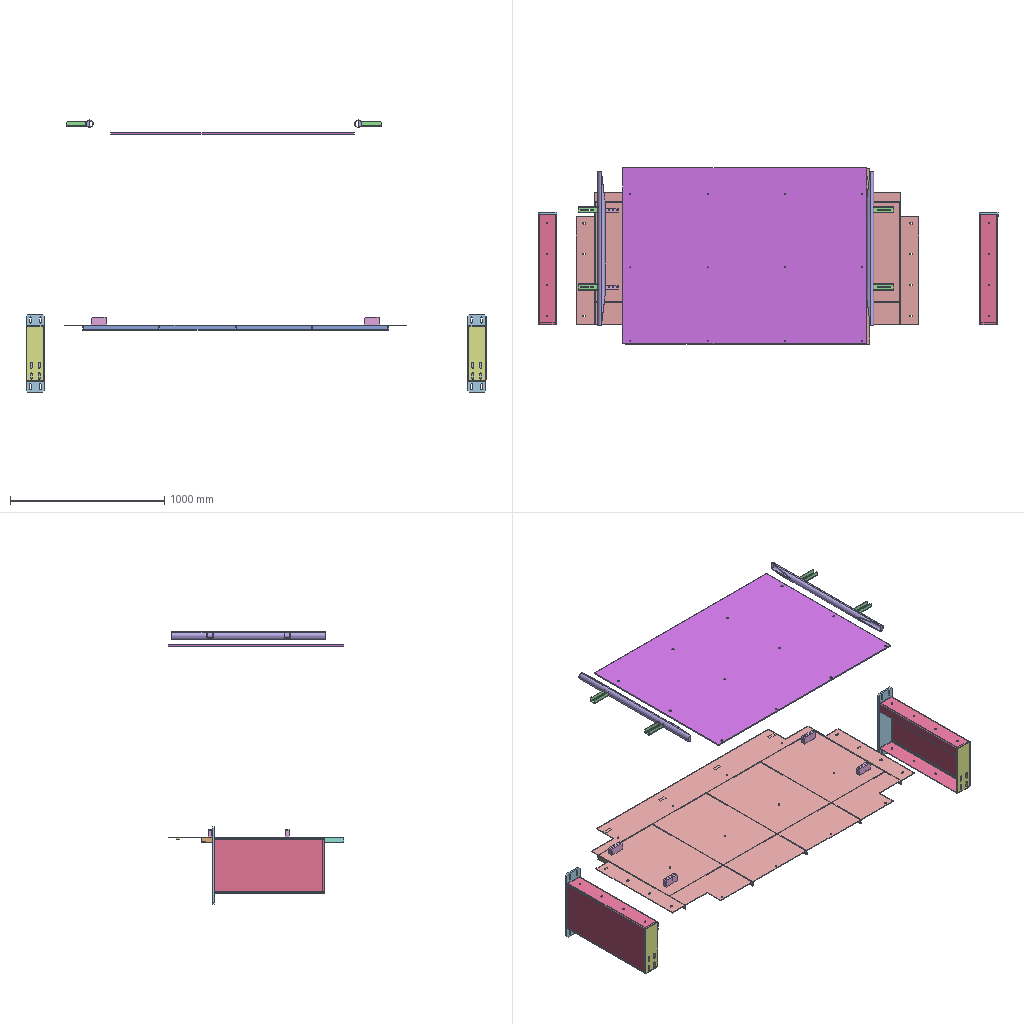Assembly | SolidWorks | 16 different items | 40 placed | box 2982 x 1140 x 1764 mm
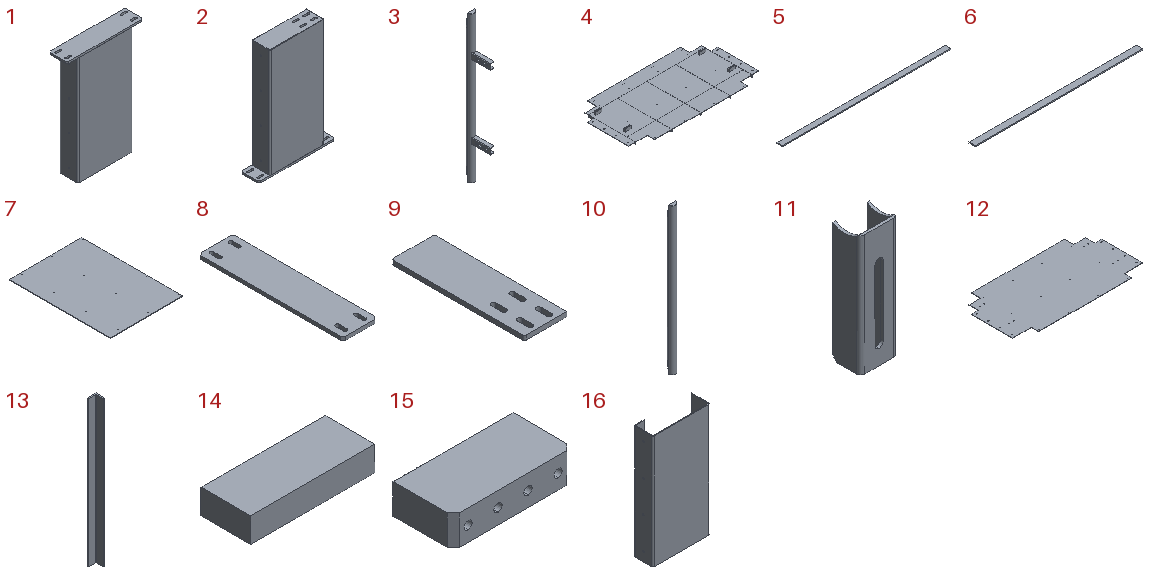Parts list (item | name | quantity | parent item | size | volume | features):
1 | (subassembly) | x1 | - | 500 x 120 x 728 mm | 2972079 mm3 | -
2 | (subassembly) | x1 | - | 500 x 120 x 728 mm | 2972079 mm3 | -
3 | (subassembly) | x2 | - | 48.3 x 173.3 x 1000 mm | 446491 mm3 | -
4 | (subassembly) | x1 | - | 2220 x 1140 x 84 mm | 11289815 mm3 | features CompositeCurve 8
5 | - | x3 | in 4 | 925 x 30 x 5 mm | 138750 mm3 | features Extrusion 1
6 | - | x2 | in 4 | 800 x 30 x 5 mm | 120000 mm3 | features Extrusion 1
7 | - | x1 | - | 1140 x 1580 x 8 mm | 14401036 mm3 | features ICE 2, Extrusion 1
8 | - | x2 | in 1, 2 | 120 x 500 x 12 mm | 694381 mm3 | features Chamfer 1, Extrusion 1, ICE 1
9 | - | x2 | in 1, 2 | 112 x 352 x 12 mm | 449676 mm3 | features Extrusion 1, Fillet 1
10 | - | x2 | in 3 | 48.3 x 48.3 x 1000 mm | 380976 mm3 | features Extrusion 1, ICE 1, Shell 1
11 | - | x4 | in 3 | 40 x 30 x 130 mm | 32768 mm3 | features ICE 2, Chamfer 1, Extrusion 1
12 | - | x1 | in 4 | 2220 x 1140 x 4 mm | 9243673 mm3 | features Extrusion 1, ICE 1
13 | - | x8 | in 4 | 30 x 30 x 490 mm | 110181 mm3 | features Extrusion 1
14 | - | x4 | in 4 | 50 x 20 x 10 mm | 10000 mm3 | features Extrusion 1
15 | - | x4 | in 4 | 100 x 50 x 25 mm | 117112 mm3 | features Chamfer 1, Extrusion 1, HoleWzd 1
16 | - | x2 | in 1, 2 | 360 x 120 x 716 mm | 1828022 mm3 | features Extrusion 1, ICE 1
Mates (type | each side: item.copy, entity, surface, feature):
In the top assembly
Coincident | 12.1 face plane Boss-Extrude1 | 7.1 face plane Boss-Extrude1
Coincident | 12.1 edge | 7.1 face cylinder Cut-Extrude1
Concentric | 12.1 face cylinder Cut-Extrude1 | 7.1 face cylinder Cut-Extrude1
Coincident | 15.1 face plane Boss-Extrude1 | 11.1 face plane Boss-Extrude1
Slot | 15.1 face cylinder M8 Tapped Hole1 | 11.1 face cylinder Cut-Extrude2 | 2 times
Coincident | 15.2 face plane Boss-Extrude1 | 11.2 face plane Boss-Extrude1
Slot | 11.2 face plane Cut-Extrude2 | 15.2 face cylinder M8 Tapped Hole1
Slot | 15.2 face cylinder M8 Tapped Hole1 | 11.2 face plane Cut-Extrude2
Coincident | 12.1 face plane Boss-Extrude1 | 16.1 face plane Boss-Extrude1
Coincident | 12.1 face plane Boss-Extrude1 | 16.2 face plane Boss-Extrude1
Slot | 16.1 face cylinder Cut-Extrude1 | 12.1 face cylinder Cut-Extrude1 | 2 times
Slot | 12.1 face plane Cut-Extrude1 | 16.2 face cylinder Cut-Extrude1 | 2 times
In subassembly 4
Coincident | 12.2 face plane Boss-Extrude1 | 6.1 face plane Boss-Extrude1 | 2 times
Coincident | 12.2 face plane Boss-Extrude1 | 6.1 edge
Coincident | 12.2 face plane Boss-Extrude1 | 5.1 face plane Boss-Extrude1
Coincident | 12.2 edge | 5.1 face plane Boss-Extrude1
Coincident | 12.2 face plane Boss-Extrude1 | 5.2 face plane Boss-Extrude1
Coincident | 12.2 face plane Boss-Extrude1 | 5.3 face plane Boss-Extrude1
Coincident | 6.1 face plane Boss-Extrude1 | 5.3 face plane Boss-Extrude1
Coincident | 5.2 face plane Boss-Extrude1 | 5.3 face plane Boss-Extrude1
DistanceDim | 5.3 face plane Boss-Extrude1 | 5.2 face plane Boss-Extrude1
DistanceDim | 5.2 face plane Boss-Extrude1 | 5.1 face plane Boss-Extrude1
DistanceDim | 6.1 face plane Boss-Extrude1 | 5.3 face plane Boss-Extrude1
Coincident | 12.2 face plane Boss-Extrude1 | 6.2 face plane Boss-Extrude1
Coincident | 5.1 face plane Boss-Extrude1 | 6.2 face plane Boss-Extrude1
DistanceDim | 5.1 face plane Boss-Extrude1 | 6.2 face plane Boss-Extrude1
Coincident | 12.2 face plane Boss-Extrude1 | 13.1 face plane Boss-Extrude1
Coincident | 6.1 face plane Boss-Extrude1 | 13.1 face plane Boss-Extrude1 | 2 times
Coincident | 13.1 face plane Boss-Extrude1 | 13.2 face plane Boss-Extrude1
Coincident | 5.2 face plane Boss-Extrude1 | 13.2 face plane Boss-Extrude1
Coincident | 12.2 face plane Boss-Extrude1 | 13.2 face plane Boss-Extrude1
Coincident | 13.3 face plane Boss-Extrude1 | 13.2 face plane Boss-Extrude1
Coincident | 13.3 face plane Boss-Extrude1 | 5.1 face plane Boss-Extrude1
Coincident | 12.2 face plane Boss-Extrude1 | 13.3 face plane Boss-Extrude1
Coincident | 13.3 face plane Boss-Extrude1 | 13.4 face plane Boss-Extrude1
Coincident | 6.2 face plane Boss-Extrude1 | 13.4 face plane Boss-Extrude1
Coincident | 12.2 face plane Boss-Extrude1 | 13.4 face plane Boss-Extrude1
Coincident | 12.2 face plane Boss-Extrude1 | 13.5 face plane Boss-Extrude1
Coincident | 5.1 face plane Boss-Extrude1 | 13.5 face plane Boss-Extrude1
DistanceDim | 13.5 face plane Boss-Extrude1 | 13.4 face plane Boss-Extrude1
Coincident | 13.5 face plane Boss-Extrude1 | 13.6 face plane Boss-Extrude1
Coincident | 5.1 face plane Boss-Extrude1 | 13.6 face plane Boss-Extrude1
Coincident | 12.2 face plane Boss-Extrude1 | 13.6 face plane Boss-Extrude1
Coincident | 13.6 face plane Boss-Extrude1 | 13.7 face plane Boss-Extrude1
Coincident | 5.2 face plane Boss-Extrude1 | 13.7 face plane Boss-Extrude1
Coincident | 12.2 face plane Boss-Extrude1 | 13.7 face plane Boss-Extrude1
Coincident | 13.8 face plane Boss-Extrude1 | 13.7 face plane Boss-Extrude1
Coincident | 5.3 face plane Boss-Extrude1 | 13.8 face plane Boss-Extrude1
Coincident | 12.2 face plane Boss-Extrude1 | 13.8 face plane Boss-Extrude1
Coincident | 12.2 face plane Boss-Extrude1 | 14.1 face plane Boss-Extrude1
Coincident | 14.1 face plane Boss-Extrude1 | 14.2 face plane Boss-Extrude1
Coincident | 14.1 face plane Boss-Extrude1 | 14.3 edge
Coincident | 14.4 face plane Boss-Extrude1 | 14.3 face plane Boss-Extrude1
Coincident | 12.2 face plane Boss-Extrude1 | 14.2 face plane Boss-Extrude1
Coincident | 12.2 face plane Boss-Extrude1 | 14.3 face plane Boss-Extrude1
Coincident | 12.2 face plane Boss-Extrude1 | 14.4 face plane Boss-Extrude1
Concentric | 12.2 edge | 15.3 face cylinder M8 Tapped Hole1 | 2 times
Concentric | 12.2 edge | 15.4 edge | 2 times
Concentric | 12.2 face cylinder Cut-Extrude1 | 15.5 face cylinder M8 Tapped Hole1
Concentric | 12.2 edge | 15.5 edge
Concentric | 12.2 face cylinder Cut-Extrude1 | 15.6 face cylinder M8 Tapped Hole1 | 2 times
Coincident | 12.2 face plane Boss-Extrude1 | 15.3 face plane Boss-Extrude1
Coincident | 12.2 face plane Boss-Extrude1 | 15.4 face plane Boss-Extrude1
Coincident | 12.2 face plane Boss-Extrude1 | 15.6 face plane Boss-Extrude1
Coincident | 12.2 face plane Boss-Extrude1 | 15.5 face plane Boss-Extrude1
DistanceDim | 14.2 face plane Boss-Extrude1 | 12.2 face plane Boss-Extrude1
DistanceDim | 14.4 face plane Boss-Extrude1 | 12.2 face plane Boss-Extrude1
DistanceDim | 14.1 face plane Boss-Extrude1 | 14.2 face plane Boss-Extrude1
DistanceDim | 14.3 face plane Boss-Extrude1 | 14.1 face plane Boss-Extrude1
In subassembly 3
Concentric | 10.1 face cylinder Boss-Extrude1 | 11.3 face cylinder Cut-Extrude1
Concentric | 10.1 face cylinder Boss-Extrude1 | 11.4 face cylinder Cut-Extrude1
Parallel | 11.3 face plane Boss-Extrude1 | 3.1 plane
Parallel | 11.3 face plane Boss-Extrude1 | 11.4 face plane Boss-Extrude1
DistanceDim | 11.4 face plane Boss-Extrude1 | 11.3 face plane Boss-Extrude1
DistanceDim | 11.4 face plane Boss-Extrude1 | 10.1 face plane Boss-Extrude1
In subassembly 1
Coincident | 16.3 face plane Boss-Extrude1 | 8.1 face plane Boss-Extrude1
Width | 8.1 face plane Boss-Extrude1 | 8.1 face plane Boss-Extrude1 | 16.3 face plane Boss-Extrude1 | 16.3 face plane Boss-Extrude1 | 2 times
Coincident | 16.3 face plane Boss-Extrude1 | 9.1 face plane Boss-Extrude1 | 3 times
In subassembly 2
Coincident | 16.3 face plane Boss-Extrude1 | 9.1 face plane Boss-Extrude1 | 2 times
Coincident | 16.3 face plane Boss-Extrude1 | 9.1 edge
Coincident | 16.3 face plane Boss-Extrude1 | 8.1 face plane Boss-Extrude1
DistanceDim | 16.3 face plane Boss-Extrude1 | 8.1 face plane Boss-Extrude1
Width | 16.3 face plane Boss-Extrude1 | 16.3 face plane Boss-Extrude1 | 8.1 face plane Boss-Extrude1 | 8.1 face plane Boss-Extrude1